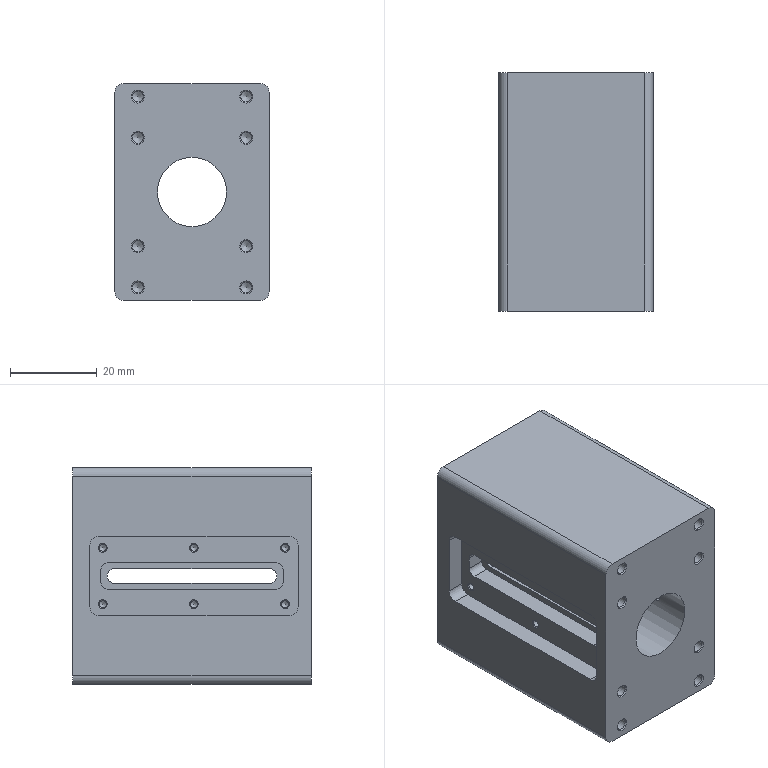Part | STEP file | Coupler cavity | 1 solid | 135 faces | box 35.5 x 55 x 50 mm | volume 76376 mm3 | cylinder 53 | cone 48 | plane 34 | commonest cylinder face diameters 3 x16 1.6 x12 2.5 x12 4 x12 16 x1